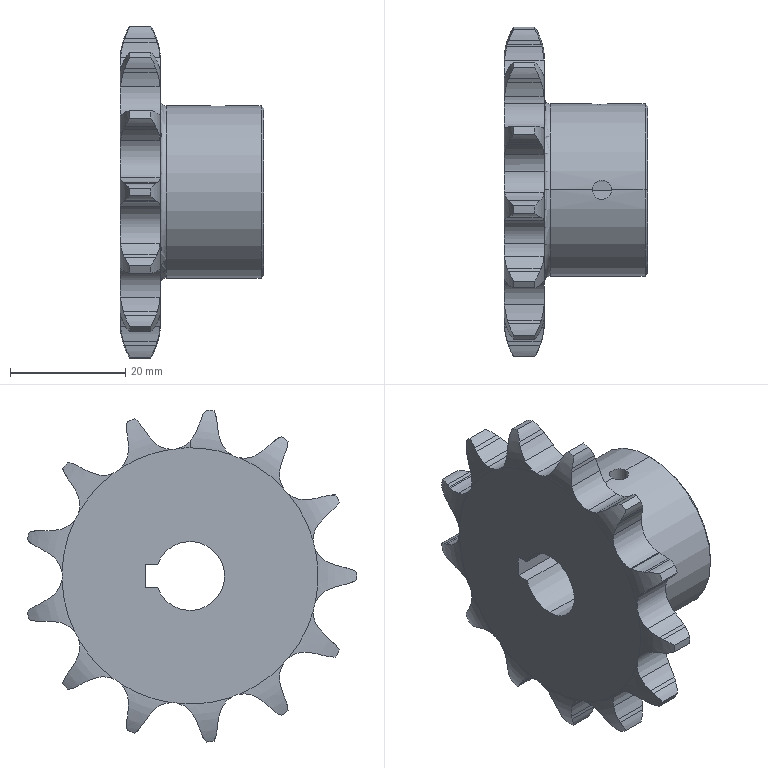Part | SolidWorks | features HoleWzd 2, ICE 2, Chamfer 1, CirPattern 1, Cut 1, Fillet 1, Revolution 1 | 1 solid | 158 faces | box 25.008 x 57.316 x 57.728 mm | volume 22718 mm3 | cylinder 94 | plane 32 | torus 30 | cone 2 | commonest cylinder face diameters 12.597 x28 22.269 x27 8.653 x17 58 x13 3.3 x4 12 x3